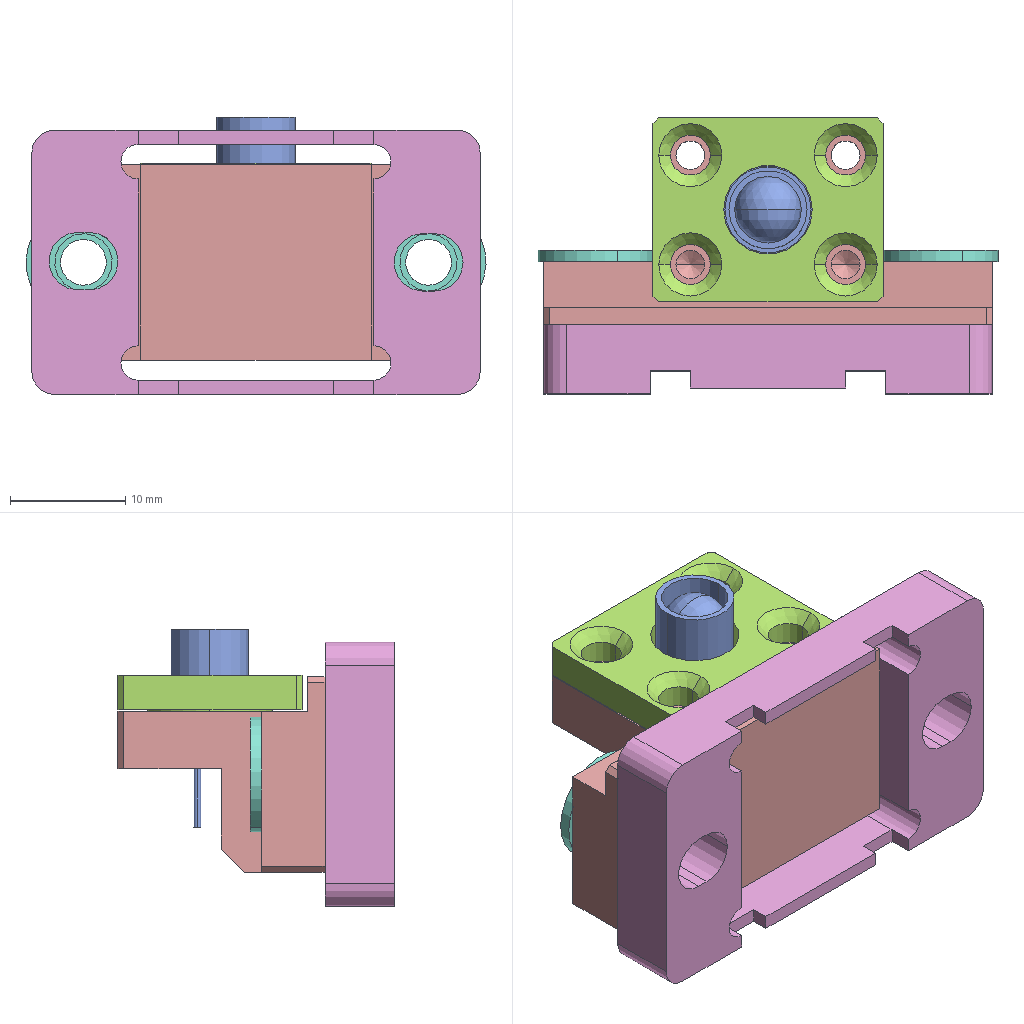Assembly | SolidWorks | 5 different items | 6 placed | box 40 x 24 x 24 mm
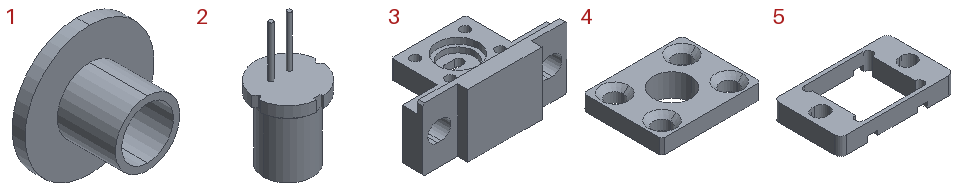Parts list (item | quantity | size | volume | features):
1 | x2 | 10 x 5.5 x 10 mm | 97.782 mm3 | features Revolution 1
2 | x1 | 8.917 x 8.972 x 17.2 mm | 386.528 mm3 | features ICE 5, Dome 1, Extrusion 1, Fillet 1, MoveFace 1
3 | x1 | 39 x 20.75 x 17 mm | 5257 mm3 | features ICE 25, MoveFace 17, Chamfer 4, 3DProfileFeature 2, Fillet 2, HoleWzd 2, Extrusion 1, MirrorPattern 1
4 | x1 | 20 x 16 x 4.6 mm | 750.45 mm3 | features Chamfer 3, Extrusion 1, ICE 1
5 | x1 | 39 x 23 x 6 mm | 2408 mm3 | features ICE 4, Cut 1, Extrusion 1, Fillet 1
Mates (type | each side: item.copy, entity, surface, feature):
Concentric | 3.1 face cylinder Boss-Extrude10 | 2.1 face cylinder Boss-Extrude2
Coincident | 3.1 face plane Boss-Extrude2 | 2.1 face plane Boss-Extrude2
Parallel | 3.1 face plane Boss-Extrude4 | 2.1 plane
Coincident | 3.1 face | assembly face | 2 times
Coincident | 3.1 select_type:0 | assembly face
Concentric | 3.1 select_type:0 | assembly face
Coincident | 3.1 face plane Mirror1 | assembly face
Parallel | 3.1 face plane Boss-Extrude6 | assembly face
Concentric | 2.1 face cylinder Boss-Extrude1 | 4.1 face cylinder Boss-Extrude1
Coincident | 2.1 face plane Boss-Extrude2 | 4.1 face plane Boss-Extrude1
Concentric | 3.1 face cylinder M3 Tapped Hole1 | 4.1 face cylinder Boss-Extrude2
Coincident | 3.1 face plane Cut-Extrude15 | 5.1 face plane Boss-Extrude1
Coincident | 3.1 face plane Boss-Extrude6 | 5.1 face plane Boss-Extrude1
Width | 3.1 face plane Boss-Extrude2 | 3.1 face plane Boss-Extrude1 | 5.1 face plane Boss-Extrude1 | 5.1 face plane Boss-Extrude1
Concentric | 3.1 select_type:24 | 1.1 face cylinder Revolve1
Coincident | 3.1 face plane Boss-Extrude13 | 1.1 face plane Revolve1
Coincident | 3.1 face plane Boss-Extrude13 | 1.2 face plane Revolve1